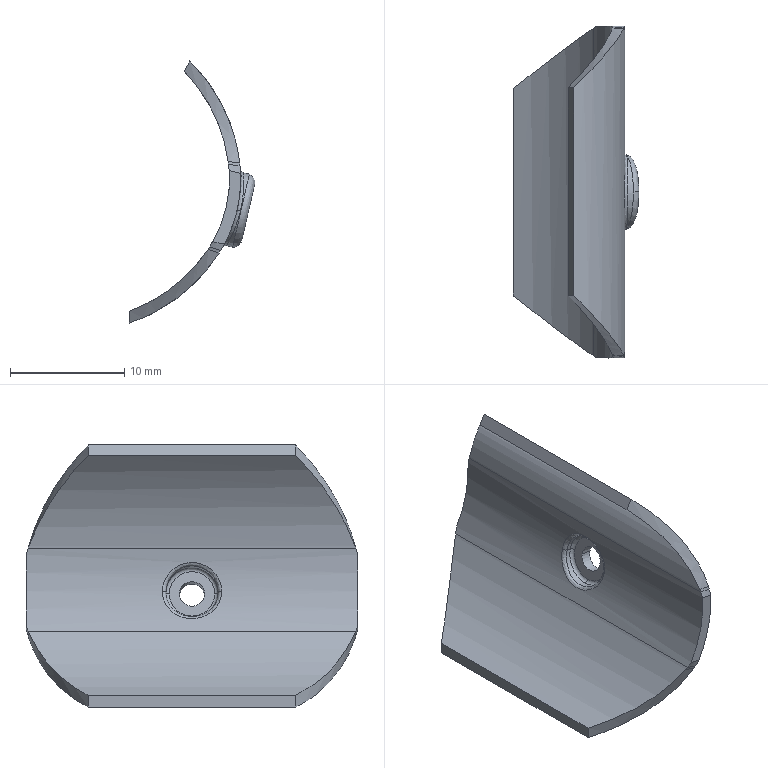Part | SolidWorks | features BaseBody 1 | 1 solid | 40 faces | box 10.992 x 29 x 22.904 mm | volume 695.627 mm3 | spline 16 | cylinder 13 | plane 6 | torus 5 | commonest cylinder face diameters 2.2 x2 4.58 x2 6.55 x2 24 x2 27.92 x2 29.89 x2